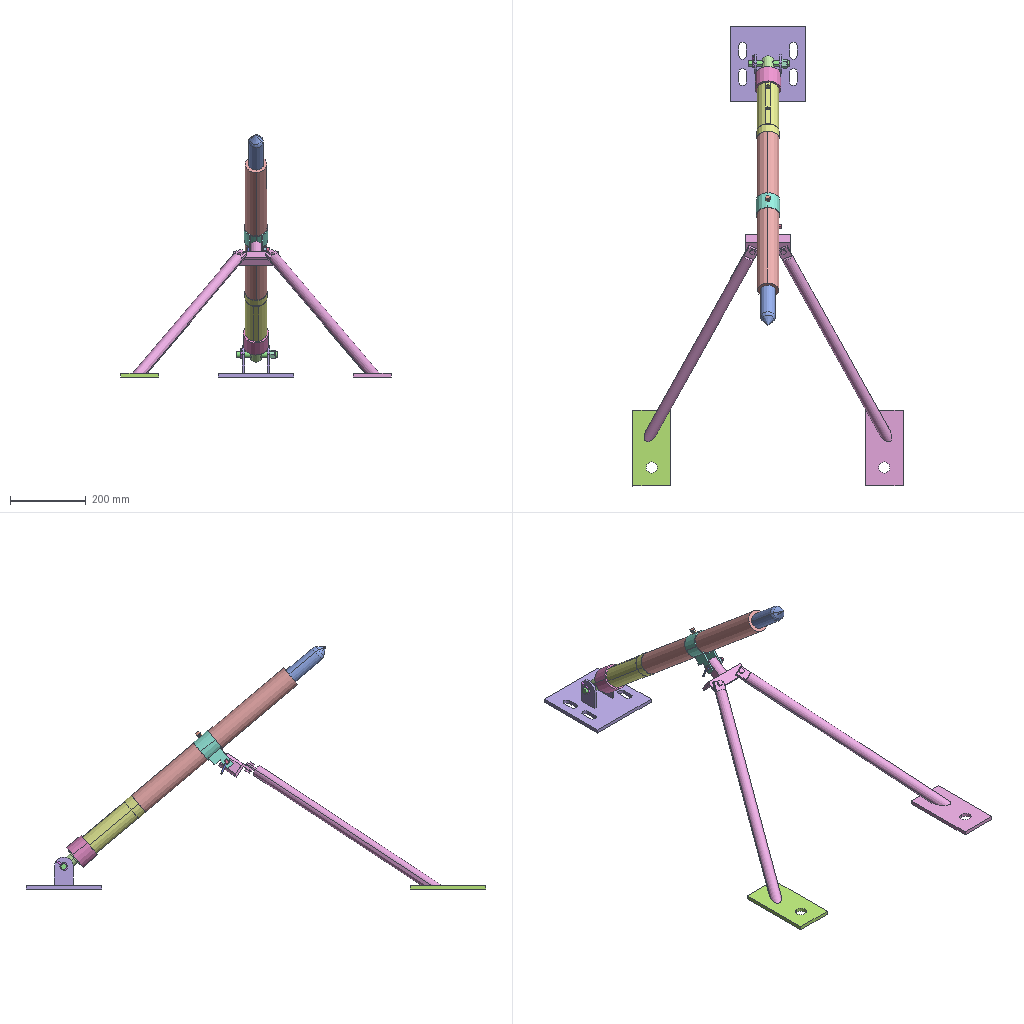Assembly | SolidWorks | 18 different items | 18 placed | box 715 x 1217 x 641 mm
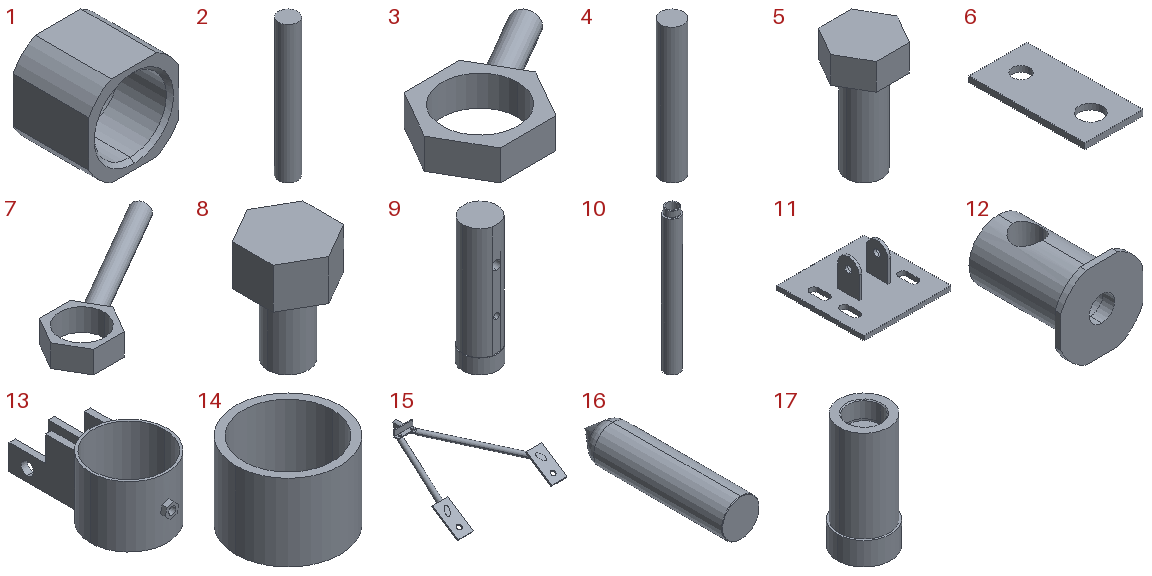Parts list (item | name | quantity | size | volume | features):
1 | - | x1 | 25 x 27 x 25 mm | 6496 mm3 | features ICE 4, Chamfer 2, Fillet 1, Revolution 1
2 | - | x1 | 15 x 15 x 107 mm | 18908 mm3 | features Extrusion 1
3 | - | x1 | 33.49 x 23.954 x 6 mm | 1120 mm3 | features Extrusion 1, ICE 1
4 | - | x1 | 10 x 10 x 60 mm | 4712 mm3 | features Extrusion 1, ICE 1
5 | - | x1 | 15 x 12.99 x 26 mm | 1882 mm3 | features Extrusion 1, ICE 1
6 | - | x1 | 50 x 100 x 5 mm | 22546 mm3 | features Extrusion 1, ICE 1
7 | - | x1 | 39.231 x 25.825 x 5 mm | 620.821 mm3 | features Extrusion 1, ICE 1
8 | - | x1 | 10.392 x 12 x 16 mm | 843.928 mm3 | features Extrusion 1, ICE 1
9 | - | x1 | 60 x 60 x 215 mm | 337627 mm3 | features ICE 6, Chamfer 1, Extrusion 1
10 | - | x1 | 58 x 58 x 550 mm | 740682 mm3 | features ICE 3, Chamfer 1, Extrusion 1, Fillet 1
11 | - | x1 | 200 x 200 x 85 mm | 407094 mm3 | features ICE 5, Extrusion 1
12 | - | x1 | 42 x 53 x 42 mm | 30095 mm3 | features ICE 8, Fillet 2, MoveFace 1, Revolution 1
13 | - | x1 | 63 x 115.25 x 50 mm | 34376 mm3 | features ICE 5, Extrusion 1
14 | - | x1 | 68 x 68 x 50 mm | 62690 mm3 | features Extrusion 1, Shell 1
15 | - | x1 | 715.381 x 770.357 x 124.108 mm | 1334452 mm3 | features ICE 15, Cut 2, MoveFace 2, Sweep 2, BossThin 1, Scale 1
16 | - | x1 | 40 x 166 x 40 mm | 188212 mm3 | features Chamfer 1, Fillet 1, Revolution 1
17 | - | x1 | 58 x 58 x 125 mm | 229241 mm3 | features ICE 5, Chamfer 2, Extrusion 1
18 | hex nut-fine pitch-style washer-grade ab gb | x1 | - | - | -
Mates (type | each side: item.copy, entity, surface, feature):
Concentric | 10.1 face cylinder Cut-Extrude2 | 16.1 face cylinder Revolve1
DistanceDim | 16.1 face plane Revolve1 | 10.1 face plane Boss-Extrude1
Concentric | 11.1 face cylinder Cut-Extrude1 | 2.1 face cylinder Boss-Extrude1
Parallel | 15.1 face plane Boss-Extrude1 | 11.1 face plane Boss-Extrude2
LimitPlanarAngleDim | 15.1 face plane Boss-Extrude1 | 13.1 face plane Boss-Extrude2
Lock | 15.1 select_type:0 | 4.1 select_type:0
Concentric | 10.1 face cylinder Boss-Extrude1 | 9.1 face cylinder Boss-Extrude1
Coincident | 10.1 face plane Boss-Extrude1 | 9.1 face plane Cut-Extrude3
Coincident | 11.1 face plane Boss-Extrude2 | 3.1 face plane Boss-Extrude1
Concentric | 2.1 face cylinder Boss-Extrude1 | 3.1 face cylinder Boss-Extrude1
Lock | 2.1 select_type:0 | 3.1 select_type:0
Tangent | 10.1 face cylinder Boss-Extrude1 | 8.1 face plane Boss-Extrude1
Concentric | 13.1 face cylinder Cut-Extrude3 | 8.1 face cylinder Boss-Extrude1
Concentric | 10.1 face cylinder Boss-Extrude1 | 13.1 face cylinder Boss-Extrude1
DistanceDim | 13.1 face plane Boss-Extrude1 | 10.1 face plane Boss-Extrude1
Concentric | 4.1 face cylinder Boss-Extrude1 | 7.1 face cylinder Boss-Extrude1
Coincident | 13.1 face plane Boss-Extrude2 | 7.1 face plane Boss-Extrude1
Lock | 4.1 select_type:0 | 7.1 select_type:0
Width | 13.1 face plane Boss-Extrude2 | 13.1 face plane Boss-Extrude2 | 15.1 face plane Boss-Extrude13 | 15.1 face plane Boss-Extrude13 | 2 times
Concentric | 13.1 face cylinder Cut-Extrude2 | 4.1 face cylinder Boss-Extrude1
Concentric | 12.1 face cylinder Revolve1 | 14.1 face cylinder Boss-Extrude1
Coincident | 12.1 face plane Revolve1 | 14.1 face plane Boss-Extrude1
Concentric | 2.1 face cylinder Boss-Extrude1 | 12.1 face cylinder Cut-Extrude6
Concentric | 9.1 face cylinder Boss-Extrude1 | 14.1 face cylinder Boss-Extrude1
Width | 11.1 face plane Boss-Extrude2 | 11.1 face plane Boss-Extrude2 | 13.1 face plane Boss-Extrude2 | 13.1 face plane Boss-Extrude2
Coincident | 9.1 face plane Boss-Extrude1 | 14.1 face plane Shell1
Parallel | 9.1 face plane Cut-Extrude1 | 8.1 face plane Boss-Extrude2
LimitPlanarAngleDim | 14.1 face plane Boss-Extrude1 | 11.1 face plane Boss-Extrude1
Lock | 2.1 select_type:0 | 12.1 select_type:0